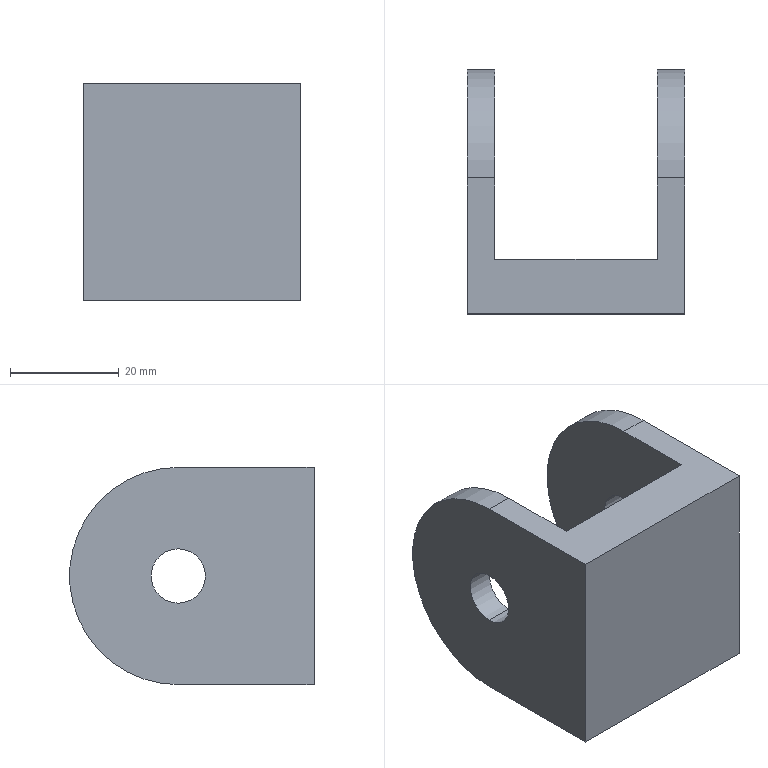Part | SolidWorks | features ICE 2, Extrusion 1, MirrorPattern 1 | 1 solid | 14 faces | box 40 x 45 x 40 mm | volume 27498 mm3 | plane 8 | cylinder 6 | commonest cylinder face diameters 10 x4 40 x2
STEP:
#1=CARTESIAN_POINT('',(15.,25.,-5.));
#2=VERTEX_POINT('',#1);
#3=CARTESIAN_POINT('',(15.,25.,5.));
#4=VERTEX_POINT('',#3);
#5=CARTESIAN_POINT('',(15.,25.,0.));
#6=DIRECTION('',(-1.,0.,0.));
#7=DIRECTION('',(0.,0.,1.));
#8=AXIS2_PLACEMENT_3D('',#5,#6,#7);
#9=CIRCLE('',#8,5.);
#10=EDGE_CURVE('',#2,#4,#9,.T.);
#11=ORIENTED_EDGE('',*,*,#10,.T.);
#12=CARTESIAN_POINT('',(20.,25.,5.));
#13=VERTEX_POINT('',#12);
#14=CARTESIAN_POINT('',(-35.,25.,5.));
#15=DIRECTION('',(1.,0.,0.));
#16=VECTOR('',#15,1000.);
#17=LINE('',#14,#16);
#18=EDGE_CURVE('',#4,#13,#17,.T.);
#19=ORIENTED_EDGE('',*,*,#18,.T.);
#20=CARTESIAN_POINT('',(20.,25.,-5.));
#21=VERTEX_POINT('',#20);
#22=CARTESIAN_POINT('',(20.,25.,0.));
#23=DIRECTION('',(-1.,0.,0.));
#24=DIRECTION('',(0.,0.,1.));
#25=AXIS2_PLACEMENT_3D('',#22,#23,#24);
#26=CIRCLE('',#25,5.);
#27=EDGE_CURVE('',#21,#13,#26,.T.);
#28=ORIENTED_EDGE('',*,*,#27,.F.);
#29=CARTESIAN_POINT('',(-35.,25.,-5.));
#30=DIRECTION('',(1.,0.,0.));
#31=VECTOR('',#30,1000.);
#32=LINE('',#29,#31);
#33=EDGE_CURVE('',#2,#21,#32,.T.);
#34=ORIENTED_EDGE('',*,*,#33,.F.);
#35=EDGE_LOOP('',(#11,#19,#28,#34));
#36=FACE_OUTER_BOUND('',#35,.T.);
#37=CARTESIAN_POINT('',(-35.,25.,0.));
#38=DIRECTION('',(1.,0.,0.));
#39=DIRECTION('',(0.,0.,-1.));
#40=AXIS2_PLACEMENT_3D('',#37,#38,#39);
#41=CYLINDRICAL_SURFACE('',#40,5.);
#42=ADVANCED_FACE('',(#36),#41,.F.);
#43=CARTESIAN_POINT('',(-20.,25.,5.));
#44=VERTEX_POINT('',#43);
#45=CARTESIAN_POINT('',(-20.,25.,-5.));
#46=VERTEX_POINT('',#45);
#47=CARTESIAN_POINT('',(-20.,25.,0.));
#48=DIRECTION('',(1.,0.,0.));
#49=DIRECTION('',(0.,0.,-1.));
#50=AXIS2_PLACEMENT_3D('',#47,#48,#49);
#51=CIRCLE('',#50,5.);
#52=EDGE_CURVE('',#44,#46,#51,.T.);
#53=ORIENTED_EDGE('',*,*,#52,.F.);
#54=CARTESIAN_POINT('',(-15.,25.,5.));
#55=VERTEX_POINT('',#54);
#56=CARTESIAN_POINT('',(-35.,25.,5.));
#57=DIRECTION('',(1.,0.,0.));
#58=VECTOR('',#57,1000.);
#59=LINE('',#56,#58);
#60=EDGE_CURVE('',#44,#55,#59,.T.);
#61=ORIENTED_EDGE('',*,*,#60,.T.);
#62=CARTESIAN_POINT('',(-15.,25.,-5.));
#63=VERTEX_POINT('',#62);
#64=CARTESIAN_POINT('',(-15.,25.,0.));
#65=DIRECTION('',(1.,0.,0.));
#66=DIRECTION('',(0.,0.,-1.));
#67=AXIS2_PLACEMENT_3D('',#64,#65,#66);
#68=CIRCLE('',#67,5.);
#69=EDGE_CURVE('',#55,#63,#68,.T.);
#70=ORIENTED_EDGE('',*,*,#69,.T.);
#71=CARTESIAN_POINT('',(-35.,25.,-5.));
#72=DIRECTION('',(1.,0.,0.));
#73=VECTOR('',#72,1000.);
#74=LINE('',#71,#73);
#75=EDGE_CURVE('',#46,#63,#74,.T.);
#76=ORIENTED_EDGE('',*,*,#75,.F.);
#77=EDGE_LOOP('',(#53,#61,#70,#76));
#78=FACE_OUTER_BOUND('',#77,.T.);
#79=CARTESIAN_POINT('',(-35.,25.,0.));
#80=DIRECTION('',(1.,0.,0.));
#81=DIRECTION('',(0.,0.,-1.));
#82=AXIS2_PLACEMENT_3D('',#79,#80,#81);
#83=CYLINDRICAL_SURFACE('',#82,5.);
#84=ADVANCED_FACE('',(#78),#83,.F.);
#85=CARTESIAN_POINT('',(-15.,10.,20.));
#86=VERTEX_POINT('',#85);
#87=CARTESIAN_POINT('',(-15.,10.,-20.));
#88=VERTEX_POINT('',#87);
#89=CARTESIAN_POINT('',(-15.,10.,20.));
#90=DIRECTION('',(0.,0.,-1.));
#91=VECTOR('',#90,1000.);
#92=LINE('',#89,#91);
#93=EDGE_CURVE('',#86,#88,#92,.T.);
#94=ORIENTED_EDGE('',*,*,#93,.F.);
#95=CARTESIAN_POINT('',(15.,10.,20.));
#96=VERTEX_POINT('',#95);
#97=CARTESIAN_POINT('',(-20.,10.,20.));
#98=DIRECTION('',(1.,0.,0.));
#99=VECTOR('',#98,1000.);
#100=LINE('',#97,#99);
#101=EDGE_CURVE('',#86,#96,#100,.T.);
#102=ORIENTED_EDGE('',*,*,#101,.T.);
#103=CARTESIAN_POINT('',(15.,10.,-20.));
#104=VERTEX_POINT('',#103);
#105=CARTESIAN_POINT('',(15.,10.,20.));
#106=DIRECTION('',(0.,0.,-1.));
#107=VECTOR('',#106,1000.);
#108=LINE('',#105,#107);
#109=EDGE_CURVE('',#96,#104,#108,.T.);
#110=ORIENTED_EDGE('',*,*,#109,.T.);
#111=CARTESIAN_POINT('',(-20.,10.,-20.));
#112=DIRECTION('',(-1.,0.,0.));
#113=VECTOR('',#112,1000.);
#114=LINE('',#111,#113);
#115=EDGE_CURVE('',#104,#88,#114,.T.);
#116=ORIENTED_EDGE('',*,*,#115,.T.);
#117=EDGE_LOOP('',(#94,#102,#110,#116));
#118=FACE_OUTER_BOUND('',#117,.T.);
#119=CARTESIAN_POINT('',(0.,10.,0.));
#120=DIRECTION('',(0.,1.,0.));
#121=DIRECTION('',(0.,0.,1.));
#122=AXIS2_PLACEMENT_3D('',#119,#120,#121);
#123=PLANE('',#122);
#124=ADVANCED_FACE('',(#118),#123,.T.);
#125=ORIENTED_EDGE('',*,*,#27,.T.);
#126=CARTESIAN_POINT('',(20.,25.,0.));
#127=DIRECTION('',(-1.,0.,0.));
#128=DIRECTION('',(0.,0.,1.));
#129=AXIS2_PLACEMENT_3D('',#126,#127,#128);
#130=CIRCLE('',#129,5.);
#131=EDGE_CURVE('',#13,#21,#130,.T.);
#132=ORIENTED_EDGE('',*,*,#131,.T.);
#133=EDGE_LOOP('',(#125,#132));
#134=FACE_BOUND('',#133,.T.);
#135=CARTESIAN_POINT('',(20.,0.,20.));
#136=VERTEX_POINT('',#135);
#137=CARTESIAN_POINT('',(20.,0.,-20.));
#138=VERTEX_POINT('',#137);
#139=CARTESIAN_POINT('',(20.,0.,-20.));
#140=DIRECTION('',(0.,0.,-1.));
#141=VECTOR('',#140,1000.);
#142=LINE('',#139,#141);
#143=EDGE_CURVE('',#136,#138,#142,.T.);
#144=ORIENTED_EDGE('',*,*,#143,.T.);
#145=CARTESIAN_POINT('',(20.,25.,-20.));
#146=VERTEX_POINT('',#145);
#147=CARTESIAN_POINT('',(20.,10.,-20.));
#148=DIRECTION('',(0.,-1.,0.));
#149=VECTOR('',#148,1000.);
#150=LINE('',#147,#149);
#151=EDGE_CURVE('',#146,#138,#150,.T.);
#152=ORIENTED_EDGE('',*,*,#151,.F.);
#153=CARTESIAN_POINT('',(20.,25.,20.));
#154=VERTEX_POINT('',#153);
#155=CARTESIAN_POINT('',(20.,25.,0.));
#156=DIRECTION('',(1.,0.,0.));
#157=DIRECTION('',(0.,0.,1.));
#158=AXIS2_PLACEMENT_3D('',#155,#156,#157);
#159=CIRCLE('',#158,20.);
#160=EDGE_CURVE('',#146,#154,#159,.T.);
#161=ORIENTED_EDGE('',*,*,#160,.T.);
#162=CARTESIAN_POINT('',(20.,10.,20.));
#163=DIRECTION('',(0.,-1.,0.));
#164=VECTOR('',#163,1000.);
#165=LINE('',#162,#164);
#166=EDGE_CURVE('',#154,#136,#165,.T.);
#167=ORIENTED_EDGE('',*,*,#166,.T.);
#168=EDGE_LOOP('',(#144,#152,#161,#167));
#169=FACE_OUTER_BOUND('',#168,.T.);
#170=CARTESIAN_POINT('',(20.,10.,-20.));
#171=DIRECTION('',(-1.,0.,0.));
#172=DIRECTION('',(0.,0.,1.));
#173=AXIS2_PLACEMENT_3D('',#170,#171,#172);
#174=PLANE('',#173);
#175=ADVANCED_FACE('',(#134,#169),#174,.F.);
#176=CARTESIAN_POINT('',(-20.,0.,-20.));
#177=VERTEX_POINT('',#176);
#178=CARTESIAN_POINT('',(-20.,0.,-20.));
#179=DIRECTION('',(-1.,0.,0.));
#180=VECTOR('',#179,1000.);
#181=LINE('',#178,#180);
#182=EDGE_CURVE('',#138,#177,#181,.T.);
#183=ORIENTED_EDGE('',*,*,#182,.T.);
#184=CARTESIAN_POINT('',(-20.,25.,-20.));
#185=VERTEX_POINT('',#184);
#186=CARTESIAN_POINT('',(-20.,10.,-20.));
#187=DIRECTION('',(0.,-1.,0.));
#188=VECTOR('',#187,1000.);
#189=LINE('',#186,#188);
#190=EDGE_CURVE('',#185,#177,#189,.T.);
#191=ORIENTED_EDGE('',*,*,#190,.F.);
#192=CARTESIAN_POINT('',(-15.,25.,-20.));
#193=VERTEX_POINT('',#192);
#194=CARTESIAN_POINT('',(-15.,25.,-20.));
#195=DIRECTION('',(-1.,0.,0.));
#196=VECTOR('',#195,1000.);
#197=LINE('',#194,#196);
#198=EDGE_CURVE('',#193,#185,#197,.T.);
#199=ORIENTED_EDGE('',*,*,#198,.F.);
#200=CARTESIAN_POINT('',(-15.,10.,-20.));
#201=DIRECTION('',(0.,1.,0.));
#202=VECTOR('',#201,1000.);
#203=LINE('',#200,#202);
#204=EDGE_CURVE('',#88,#193,#203,.T.);
#205=ORIENTED_EDGE('',*,*,#204,.F.);
#206=ORIENTED_EDGE('',*,*,#115,.F.);
#207=CARTESIAN_POINT('',(15.,25.,-20.));
#208=VERTEX_POINT('',#207);
#209=CARTESIAN_POINT('',(15.,10.,-20.));
#210=DIRECTION('',(0.,1.,0.));
#211=VECTOR('',#210,1000.);
#212=LINE('',#209,#211);
#213=EDGE_CURVE('',#104,#208,#212,.T.);
#214=ORIENTED_EDGE('',*,*,#213,.T.);
#215=CARTESIAN_POINT('',(15.,25.,-20.));
#216=DIRECTION('',(1.,0.,0.));
#217=VECTOR('',#216,1000.);
#218=LINE('',#215,#217);
#219=EDGE_CURVE('',#208,#146,#218,.T.);
#220=ORIENTED_EDGE('',*,*,#219,.T.);
#221=ORIENTED_EDGE('',*,*,#151,.T.);
#222=EDGE_LOOP('',(#183,#191,#199,#205,#206,#214,#220,#221));
#223=FACE_OUTER_BOUND('',#222,.T.);
#224=CARTESIAN_POINT('',(-20.,10.,-20.));
#225=DIRECTION('',(0.,0.,1.));
#226=DIRECTION('',(1.,0.,0.));
#227=AXIS2_PLACEMENT_3D('',#224,#225,#226);
#228=PLANE('',#227);
#229=ADVANCED_FACE('',(#223),#228,.F.);
#230=CARTESIAN_POINT('',(-20.,25.,0.));
#231=DIRECTION('',(1.,0.,0.));
#232=DIRECTION('',(0.,0.,-1.));
#233=AXIS2_PLACEMENT_3D('',#230,#231,#232);
#234=CIRCLE('',#233,5.);
#235=EDGE_CURVE('',#46,#44,#234,.T.);
#236=ORIENTED_EDGE('',*,*,#235,.T.);
#237=ORIENTED_EDGE('',*,*,#52,.T.);
#238=EDGE_LOOP('',(#236,#237));
#239=FACE_BOUND('',#238,.T.);
#240=CARTESIAN_POINT('',(-20.,0.,20.));
#241=VERTEX_POINT('',#240);
#242=CARTESIAN_POINT('',(-20.,0.,-20.));
#243=DIRECTION('',(0.,0.,1.));
#244=VECTOR('',#243,1000.);
#245=LINE('',#242,#244);
#246=EDGE_CURVE('',#177,#241,#245,.T.);
#247=ORIENTED_EDGE('',*,*,#246,.T.);
#248=CARTESIAN_POINT('',(-20.,25.,20.));
#249=VERTEX_POINT('',#248);
#250=CARTESIAN_POINT('',(-20.,10.,20.));
#251=DIRECTION('',(0.,-1.,0.));
#252=VECTOR('',#251,1000.);
#253=LINE('',#250,#252);
#254=EDGE_CURVE('',#249,#241,#253,.T.);
#255=ORIENTED_EDGE('',*,*,#254,.F.);
#256=CARTESIAN_POINT('',(-20.,25.,0.));
#257=DIRECTION('',(1.,0.,0.));
#258=DIRECTION('',(0.,0.,1.));
#259=AXIS2_PLACEMENT_3D('',#256,#257,#258);
#260=CIRCLE('',#259,20.);
#261=EDGE_CURVE('',#185,#249,#260,.T.);
#262=ORIENTED_EDGE('',*,*,#261,.F.);
#263=ORIENTED_EDGE('',*,*,#190,.T.);
#264=EDGE_LOOP('',(#247,#255,#262,#263));
#265=FACE_OUTER_BOUND('',#264,.T.);
#266=CARTESIAN_POINT('',(-20.,10.,-20.));
#267=DIRECTION('',(1.,0.,0.));
#268=DIRECTION('',(0.,0.,-1.));
#269=AXIS2_PLACEMENT_3D('',#266,#267,#268);
#270=PLANE('',#269);
#271=ADVANCED_FACE('',(#239,#265),#270,.F.);
#272=CARTESIAN_POINT('',(-20.,0.,20.));
#273=DIRECTION('',(1.,0.,0.));
#274=VECTOR('',#273,1000.);
#275=LINE('',#272,#274);
#276=EDGE_CURVE('',#241,#136,#275,.T.);
#277=ORIENTED_EDGE('',*,*,#276,.T.);
#278=ORIENTED_EDGE('',*,*,#166,.F.);
#279=CARTESIAN_POINT('',(15.,25.,20.));
#280=VERTEX_POINT('',#279);
#281=CARTESIAN_POINT('',(15.,25.,20.));
#282=DIRECTION('',(1.,0.,0.));
#283=VECTOR('',#282,1000.);
#284=LINE('',#281,#283);
#285=EDGE_CURVE('',#280,#154,#284,.T.);
#286=ORIENTED_EDGE('',*,*,#285,.F.);
#287=CARTESIAN_POINT('',(15.,10.,20.));
#288=DIRECTION('',(0.,-1.,0.));
#289=VECTOR('',#288,1000.);
#290=LINE('',#287,#289);
#291=EDGE_CURVE('',#280,#96,#290,.T.);
#292=ORIENTED_EDGE('',*,*,#291,.T.);
#293=ORIENTED_EDGE('',*,*,#101,.F.);
#294=CARTESIAN_POINT('',(-15.,25.,20.));
#295=VERTEX_POINT('',#294);
#296=CARTESIAN_POINT('',(-15.,10.,20.));
#297=DIRECTION('',(0.,-1.,0.));
#298=VECTOR('',#297,1000.);
#299=LINE('',#296,#298);
#300=EDGE_CURVE('',#295,#86,#299,.T.);
#301=ORIENTED_EDGE('',*,*,#300,.F.);
#302=CARTESIAN_POINT('',(-15.,25.,20.));
#303=DIRECTION('',(-1.,0.,0.));
#304=VECTOR('',#303,1000.);
#305=LINE('',#302,#304);
#306=EDGE_CURVE('',#295,#249,#305,.T.);
#307=ORIENTED_EDGE('',*,*,#306,.T.);
#308=ORIENTED_EDGE('',*,*,#254,.T.);
#309=EDGE_LOOP('',(#277,#278,#286,#292,#293,#301,#307,#308));
#310=FACE_OUTER_BOUND('',#309,.T.);
#311=CARTESIAN_POINT('',(-20.,10.,20.));
#312=DIRECTION('',(0.,0.,-1.));
#313=DIRECTION('',(-1.,0.,0.));
#314=AXIS2_PLACEMENT_3D('',#311,#312,#313);
#315=PLANE('',#314);
#316=ADVANCED_FACE('',(#310),#315,.F.);
#317=ORIENTED_EDGE('',*,*,#143,.F.);
#318=ORIENTED_EDGE('',*,*,#276,.F.);
#319=ORIENTED_EDGE('',*,*,#246,.F.);
#320=ORIENTED_EDGE('',*,*,#182,.F.);
#321=EDGE_LOOP('',(#317,#318,#319,#320));
#322=FACE_OUTER_BOUND('',#321,.T.);
#323=CARTESIAN_POINT('',(0.,0.,0.));
#324=DIRECTION('',(0.,1.,0.));
#325=DIRECTION('',(0.,0.,1.));
#326=AXIS2_PLACEMENT_3D('',#323,#324,#325);
#327=PLANE('',#326);
#328=ADVANCED_FACE('',(#322),#327,.F.);
#329=ORIENTED_EDGE('',*,*,#160,.F.);
#330=ORIENTED_EDGE('',*,*,#219,.F.);
#331=CARTESIAN_POINT('',(15.,25.,0.));
#332=DIRECTION('',(1.,0.,0.));
#333=DIRECTION('',(0.,0.,1.));
#334=AXIS2_PLACEMENT_3D('',#331,#332,#333);
#335=CIRCLE('',#334,20.);
#336=EDGE_CURVE('',#208,#280,#335,.T.);
#337=ORIENTED_EDGE('',*,*,#336,.T.);
#338=ORIENTED_EDGE('',*,*,#285,.T.);
#339=EDGE_LOOP('',(#329,#330,#337,#338));
#340=FACE_OUTER_BOUND('',#339,.T.);
#341=CARTESIAN_POINT('',(15.,25.,0.));
#342=DIRECTION('',(1.,0.,0.));
#343=DIRECTION('',(0.,0.,-1.));
#344=AXIS2_PLACEMENT_3D('',#341,#342,#343);
#345=CYLINDRICAL_SURFACE('',#344,20.);
#346=ADVANCED_FACE('',(#340),#345,.T.);
#347=ORIENTED_EDGE('',*,*,#10,.F.);
#348=CARTESIAN_POINT('',(15.,25.,0.));
#349=DIRECTION('',(-1.,0.,0.));
#350=DIRECTION('',(0.,0.,1.));
#351=AXIS2_PLACEMENT_3D('',#348,#349,#350);
#352=CIRCLE('',#351,5.);
#353=EDGE_CURVE('',#4,#2,#352,.T.);
#354=ORIENTED_EDGE('',*,*,#353,.F.);
#355=EDGE_LOOP('',(#347,#354));
#356=FACE_BOUND('',#355,.T.);
#357=ORIENTED_EDGE('',*,*,#109,.F.);
#358=ORIENTED_EDGE('',*,*,#291,.F.);
#359=ORIENTED_EDGE('',*,*,#336,.F.);
#360=ORIENTED_EDGE('',*,*,#213,.F.);
#361=EDGE_LOOP('',(#357,#358,#359,#360));
#362=FACE_OUTER_BOUND('',#361,.T.);
#363=CARTESIAN_POINT('',(15.,25.,0.));
#364=DIRECTION('',(-1.,0.,0.));
#365=DIRECTION('',(0.,0.,1.));
#366=AXIS2_PLACEMENT_3D('',#363,#364,#365);
#367=PLANE('',#366);
#368=ADVANCED_FACE('',(#356,#362),#367,.T.);
#369=ORIENTED_EDGE('',*,*,#261,.T.);
#370=ORIENTED_EDGE('',*,*,#306,.F.);
#371=CARTESIAN_POINT('',(-15.,25.,0.));
#372=DIRECTION('',(1.,0.,0.));
#373=DIRECTION('',(0.,0.,1.));
#374=AXIS2_PLACEMENT_3D('',#371,#372,#373);
#375=CIRCLE('',#374,20.);
#376=EDGE_CURVE('',#193,#295,#375,.T.);
#377=ORIENTED_EDGE('',*,*,#376,.F.);
#378=ORIENTED_EDGE('',*,*,#198,.T.);
#379=EDGE_LOOP('',(#369,#370,#377,#378));
#380=FACE_OUTER_BOUND('',#379,.T.);
#381=CARTESIAN_POINT('',(-15.,25.,0.));
#382=DIRECTION('',(-1.,0.,0.));
#383=DIRECTION('',(0.,0.,1.));
#384=AXIS2_PLACEMENT_3D('',#381,#382,#383);
#385=CYLINDRICAL_SURFACE('',#384,20.);
#386=ADVANCED_FACE('',(#380),#385,.T.);
#387=CARTESIAN_POINT('',(-15.,25.,0.));
#388=DIRECTION('',(1.,0.,0.));
#389=DIRECTION('',(0.,0.,-1.));
#390=AXIS2_PLACEMENT_3D('',#387,#388,#389);
#391=CIRCLE('',#390,5.);
#392=EDGE_CURVE('',#63,#55,#391,.T.);
#393=ORIENTED_EDGE('',*,*,#392,.F.);
#394=ORIENTED_EDGE('',*,*,#69,.F.);
#395=EDGE_LOOP('',(#393,#394));
#396=FACE_BOUND('',#395,.T.);
#397=ORIENTED_EDGE('',*,*,#93,.T.);
#398=ORIENTED_EDGE('',*,*,#204,.T.);
#399=ORIENTED_EDGE('',*,*,#376,.T.);
#400=ORIENTED_EDGE('',*,*,#300,.T.);
#401=EDGE_LOOP('',(#397,#398,#399,#400));
#402=FACE_OUTER_BOUND('',#401,.T.);
#403=CARTESIAN_POINT('',(-15.,25.,0.));
#404=DIRECTION('',(1.,0.,0.));
#405=DIRECTION('',(0.,0.,1.));
#406=AXIS2_PLACEMENT_3D('',#403,#404,#405);
#407=PLANE('',#406);
#408=ADVANCED_FACE('',(#396,#402),#407,.T.);
#409=ORIENTED_EDGE('',*,*,#60,.F.);
#410=ORIENTED_EDGE('',*,*,#235,.F.);
#411=ORIENTED_EDGE('',*,*,#75,.T.);
#412=ORIENTED_EDGE('',*,*,#392,.T.);
#413=EDGE_LOOP('',(#409,#410,#411,#412));
#414=FACE_OUTER_BOUND('',#413,.T.);
#415=CARTESIAN_POINT('',(-35.,25.,0.));
#416=DIRECTION('',(1.,0.,0.));
#417=DIRECTION('',(0.,0.,-1.));
#418=AXIS2_PLACEMENT_3D('',#415,#416,#417);
#419=CYLINDRICAL_SURFACE('',#418,5.);
#420=ADVANCED_FACE('',(#414),#419,.F.);
#421=ORIENTED_EDGE('',*,*,#18,.F.);
#422=ORIENTED_EDGE('',*,*,#353,.T.);
#423=ORIENTED_EDGE('',*,*,#33,.T.);
#424=ORIENTED_EDGE('',*,*,#131,.F.);
#425=EDGE_LOOP('',(#421,#422,#423,#424));
#426=FACE_OUTER_BOUND('',#425,.T.);
#427=CARTESIAN_POINT('',(-35.,25.,0.));
#428=DIRECTION('',(1.,0.,0.));
#429=DIRECTION('',(0.,0.,-1.));
#430=AXIS2_PLACEMENT_3D('',#427,#428,#429);
#431=CYLINDRICAL_SURFACE('',#430,5.);
#432=ADVANCED_FACE('',(#426),#431,.F.);
#433=CLOSED_SHELL('',(#42,#84,#124,#175,#229,#271,#316,#328,#346,#368,#386,#408,#420,#432));
#434=MANIFOLD_SOLID_BREP('',#433);
#435=CARTESIAN_POINT('',(0.,0.,0.));
#436=DIRECTION('',(0.,0.,1.));
#437=DIRECTION('',(1.,0.,0.));
#438=AXIS2_PLACEMENT_3D('',#435,#436,#437);
#439=(LENGTH_UNIT()NAMED_UNIT(*)SI_UNIT(.MILLI.,.METRE.));
#440=UNCERTAINTY_MEASURE_WITH_UNIT(LENGTH_MEASURE(0.00001),#439,'','');
#441=(NAMED_UNIT(*)PLANE_ANGLE_UNIT()SI_UNIT($,.RADIAN.));
#442=(NAMED_UNIT(*)SI_UNIT($,.STERADIAN.)SOLID_ANGLE_UNIT());
#443=(GEOMETRIC_REPRESENTATION_CONTEXT(3)GLOBAL_UNCERTAINTY_ASSIGNED_CONTEXT((#440))GLOBAL_UNIT_ASSIGNED_CONTEXT((#439,#441,#442))REPRESENTATION_CONTEXT('',''));
#444=ADVANCED_BREP_SHAPE_REPRESENTATION('',(#434,#438),#443);